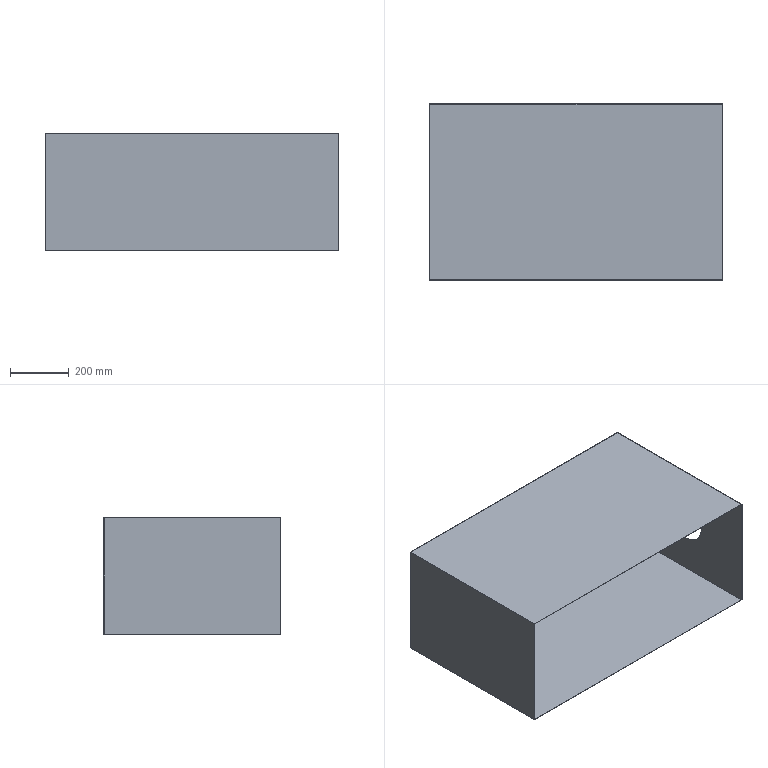Part | SolidWorks | features Cut 1, Extrusion 1, ICE 1 | 1 solid | 13 faces | box 1000 x 600 x 400 mm | volume 2057133 mm3 | plane 11 | cylinder 2 | commonest cylinder face diameters 150 x2
STEP:
#1=CARTESIAN_POINT('',(499.,270.,75.));
#2=VERTEX_POINT('',#1);
#3=CARTESIAN_POINT('',(499.,270.,-75.));
#4=VERTEX_POINT('',#3);
#5=CARTESIAN_POINT('',(499.,270.,0.));
#6=DIRECTION('',(1.,0.,0.));
#7=DIRECTION('',(0.,0.,-1.));
#8=AXIS2_PLACEMENT_3D('',#5,#6,#7);
#9=CIRCLE('',#8,75.);
#10=EDGE_CURVE('',#2,#4,#9,.T.);
#11=ORIENTED_EDGE('',*,*,#10,.F.);
#12=CARTESIAN_POINT('',(500.,270.,75.));
#13=VERTEX_POINT('',#12);
#14=CARTESIAN_POINT('',(450.,270.,75.));
#15=DIRECTION('',(1.,0.,0.));
#16=VECTOR('',#15,1000.);
#17=LINE('',#14,#16);
#18=EDGE_CURVE('',#2,#13,#17,.T.);
#19=ORIENTED_EDGE('',*,*,#18,.T.);
#20=CARTESIAN_POINT('',(500.,270.,-75.));
#21=VERTEX_POINT('',#20);
#22=CARTESIAN_POINT('',(500.,270.,0.));
#23=DIRECTION('',(1.,0.,0.));
#24=DIRECTION('',(0.,0.,-1.));
#25=AXIS2_PLACEMENT_3D('',#22,#23,#24);
#26=CIRCLE('',#25,75.);
#27=EDGE_CURVE('',#13,#21,#26,.T.);
#28=ORIENTED_EDGE('',*,*,#27,.T.);
#29=CARTESIAN_POINT('',(450.,270.,-75.));
#30=DIRECTION('',(1.,0.,0.));
#31=VECTOR('',#30,1000.);
#32=LINE('',#29,#31);
#33=EDGE_CURVE('',#4,#21,#32,.T.);
#34=ORIENTED_EDGE('',*,*,#33,.F.);
#35=EDGE_LOOP('',(#11,#19,#28,#34));
#36=FACE_OUTER_BOUND('',#35,.T.);
#37=CARTESIAN_POINT('',(450.,270.,0.));
#38=DIRECTION('',(1.,0.,0.));
#39=DIRECTION('',(0.,0.,-1.));
#40=AXIS2_PLACEMENT_3D('',#37,#38,#39);
#41=CYLINDRICAL_SURFACE('',#40,75.);
#42=ADVANCED_FACE('',(#36),#41,.F.);
#43=CARTESIAN_POINT('',(500.,270.,0.));
#44=DIRECTION('',(1.,0.,0.));
#45=DIRECTION('',(0.,0.,-1.));
#46=AXIS2_PLACEMENT_3D('',#43,#44,#45);
#47=CIRCLE('',#46,75.);
#48=EDGE_CURVE('',#21,#13,#47,.T.);
#49=ORIENTED_EDGE('',*,*,#48,.F.);
#50=ORIENTED_EDGE('',*,*,#27,.F.);
#51=EDGE_LOOP('',(#49,#50));
#52=FACE_BOUND('',#51,.T.);
#53=CARTESIAN_POINT('',(500.,0.,200.));
#54=VERTEX_POINT('',#53);
#55=CARTESIAN_POINT('',(500.,0.,-200.));
#56=VERTEX_POINT('',#55);
#57=CARTESIAN_POINT('',(500.,0.,-200.));
#58=DIRECTION('',(0.,0.,-1.));
#59=VECTOR('',#58,1000.);
#60=LINE('',#57,#59);
#61=EDGE_CURVE('',#54,#56,#60,.T.);
#62=ORIENTED_EDGE('',*,*,#61,.T.);
#63=CARTESIAN_POINT('',(500.,600.,-200.));
#64=VERTEX_POINT('',#63);
#65=CARTESIAN_POINT('',(500.,600.,-200.));
#66=DIRECTION('',(0.,-1.,0.));
#67=VECTOR('',#66,1000.);
#68=LINE('',#65,#67);
#69=EDGE_CURVE('',#64,#56,#68,.T.);
#70=ORIENTED_EDGE('',*,*,#69,.F.);
#71=CARTESIAN_POINT('',(500.,600.,200.));
#72=VERTEX_POINT('',#71);
#73=CARTESIAN_POINT('',(500.,600.,-200.));
#74=DIRECTION('',(0.,0.,-1.));
#75=VECTOR('',#74,1000.);
#76=LINE('',#73,#75);
#77=EDGE_CURVE('',#72,#64,#76,.T.);
#78=ORIENTED_EDGE('',*,*,#77,.F.);
#79=CARTESIAN_POINT('',(500.,600.,200.));
#80=DIRECTION('',(0.,-1.,0.));
#81=VECTOR('',#80,1000.);
#82=LINE('',#79,#81);
#83=EDGE_CURVE('',#72,#54,#82,.T.);
#84=ORIENTED_EDGE('',*,*,#83,.T.);
#85=EDGE_LOOP('',(#62,#70,#78,#84));
#86=FACE_OUTER_BOUND('',#85,.T.);
#87=CARTESIAN_POINT('',(500.,600.,-200.));
#88=DIRECTION('',(-1.,0.,0.));
#89=DIRECTION('',(0.,0.,1.));
#90=AXIS2_PLACEMENT_3D('',#87,#88,#89);
#91=PLANE('',#90);
#92=ADVANCED_FACE('',(#52,#86),#91,.F.);
#93=CARTESIAN_POINT('',(-500.,0.,-200.));
#94=VERTEX_POINT('',#93);
#95=CARTESIAN_POINT('',(-500.,0.,-200.));
#96=DIRECTION('',(-1.,0.,0.));
#97=VECTOR('',#96,1000.);
#98=LINE('',#95,#97);
#99=EDGE_CURVE('',#56,#94,#98,.T.);
#100=ORIENTED_EDGE('',*,*,#99,.T.);
#101=CARTESIAN_POINT('',(-500.,600.,-200.));
#102=VERTEX_POINT('',#101);
#103=CARTESIAN_POINT('',(-500.,600.,-200.));
#104=DIRECTION('',(0.,-1.,0.));
#105=VECTOR('',#104,1000.);
#106=LINE('',#103,#105);
#107=EDGE_CURVE('',#102,#94,#106,.T.);
#108=ORIENTED_EDGE('',*,*,#107,.F.);
#109=CARTESIAN_POINT('',(-500.,600.,-200.));
#110=DIRECTION('',(-1.,0.,0.));
#111=VECTOR('',#110,1000.);
#112=LINE('',#109,#111);
#113=EDGE_CURVE('',#64,#102,#112,.T.);
#114=ORIENTED_EDGE('',*,*,#113,.F.);
#115=ORIENTED_EDGE('',*,*,#69,.T.);
#116=EDGE_LOOP('',(#100,#108,#114,#115));
#117=FACE_OUTER_BOUND('',#116,.T.);
#118=CARTESIAN_POINT('',(-500.,600.,-200.));
#119=DIRECTION('',(0.,0.,1.));
#120=DIRECTION('',(1.,0.,0.));
#121=AXIS2_PLACEMENT_3D('',#118,#119,#120);
#122=PLANE('',#121);
#123=ADVANCED_FACE('',(#117),#122,.F.);
#124=CARTESIAN_POINT('',(-500.,0.,200.));
#125=VERTEX_POINT('',#124);
#126=CARTESIAN_POINT('',(-500.,0.,-200.));
#127=DIRECTION('',(0.,0.,1.));
#128=VECTOR('',#127,1000.);
#129=LINE('',#126,#128);
#130=EDGE_CURVE('',#94,#125,#129,.T.);
#131=ORIENTED_EDGE('',*,*,#130,.T.);
#132=CARTESIAN_POINT('',(-500.,600.,200.));
#133=VERTEX_POINT('',#132);
#134=CARTESIAN_POINT('',(-500.,600.,200.));
#135=DIRECTION('',(0.,-1.,0.));
#136=VECTOR('',#135,1000.);
#137=LINE('',#134,#136);
#138=EDGE_CURVE('',#133,#125,#137,.T.);
#139=ORIENTED_EDGE('',*,*,#138,.F.);
#140=CARTESIAN_POINT('',(-500.,600.,-200.));
#141=DIRECTION('',(0.,0.,1.));
#142=VECTOR('',#141,1000.);
#143=LINE('',#140,#142);
#144=EDGE_CURVE('',#102,#133,#143,.T.);
#145=ORIENTED_EDGE('',*,*,#144,.F.);
#146=ORIENTED_EDGE('',*,*,#107,.T.);
#147=EDGE_LOOP('',(#131,#139,#145,#146));
#148=FACE_OUTER_BOUND('',#147,.T.);
#149=CARTESIAN_POINT('',(-500.,600.,-200.));
#150=DIRECTION('',(1.,0.,0.));
#151=DIRECTION('',(0.,0.,-1.));
#152=AXIS2_PLACEMENT_3D('',#149,#150,#151);
#153=PLANE('',#152);
#154=ADVANCED_FACE('',(#148),#153,.F.);
#155=CARTESIAN_POINT('',(-500.,0.,200.));
#156=DIRECTION('',(1.,0.,0.));
#157=VECTOR('',#156,1000.);
#158=LINE('',#155,#157);
#159=EDGE_CURVE('',#125,#54,#158,.T.);
#160=ORIENTED_EDGE('',*,*,#159,.T.);
#161=ORIENTED_EDGE('',*,*,#83,.F.);
#162=CARTESIAN_POINT('',(-500.,600.,200.));
#163=DIRECTION('',(1.,0.,0.));
#164=VECTOR('',#163,1000.);
#165=LINE('',#162,#164);
#166=EDGE_CURVE('',#133,#72,#165,.T.);
#167=ORIENTED_EDGE('',*,*,#166,.F.);
#168=ORIENTED_EDGE('',*,*,#138,.T.);
#169=EDGE_LOOP('',(#160,#161,#167,#168));
#170=FACE_OUTER_BOUND('',#169,.T.);
#171=CARTESIAN_POINT('',(-500.,600.,200.));
#172=DIRECTION('',(0.,0.,-1.));
#173=DIRECTION('',(-1.,0.,0.));
#174=AXIS2_PLACEMENT_3D('',#171,#172,#173);
#175=PLANE('',#174);
#176=ADVANCED_FACE('',(#170),#175,.F.);
#177=ORIENTED_EDGE('',*,*,#77,.T.);
#178=ORIENTED_EDGE('',*,*,#113,.T.);
#179=ORIENTED_EDGE('',*,*,#144,.T.);
#180=ORIENTED_EDGE('',*,*,#166,.T.);
#181=EDGE_LOOP('',(#177,#178,#179,#180));
#182=FACE_OUTER_BOUND('',#181,.T.);
#183=CARTESIAN_POINT('',(0.,600.,0.));
#184=DIRECTION('',(0.,1.,0.));
#185=DIRECTION('',(0.,0.,1.));
#186=AXIS2_PLACEMENT_3D('',#183,#184,#185);
#187=PLANE('',#186);
#188=ADVANCED_FACE('',(#182),#187,.T.);
#189=CARTESIAN_POINT('',(499.,0.,199.));
#190=VERTEX_POINT('',#189);
#191=CARTESIAN_POINT('',(-499.,0.,199.));
#192=VERTEX_POINT('',#191);
#193=CARTESIAN_POINT('',(-499.,0.,199.));
#194=DIRECTION('',(-1.,0.,0.));
#195=VECTOR('',#194,1000.);
#196=LINE('',#193,#195);
#197=EDGE_CURVE('',#190,#192,#196,.T.);
#198=ORIENTED_EDGE('',*,*,#197,.F.);
#199=CARTESIAN_POINT('',(499.,0.,-199.));
#200=VERTEX_POINT('',#199);
#201=CARTESIAN_POINT('',(499.,0.,-199.));
#202=DIRECTION('',(0.,0.,1.));
#203=VECTOR('',#202,1000.);
#204=LINE('',#201,#203);
#205=EDGE_CURVE('',#200,#190,#204,.T.);
#206=ORIENTED_EDGE('',*,*,#205,.F.);
#207=CARTESIAN_POINT('',(-499.,0.,-199.));
#208=VERTEX_POINT('',#207);
#209=CARTESIAN_POINT('',(-499.,0.,-199.));
#210=DIRECTION('',(1.,0.,0.));
#211=VECTOR('',#210,1000.);
#212=LINE('',#209,#211);
#213=EDGE_CURVE('',#208,#200,#212,.T.);
#214=ORIENTED_EDGE('',*,*,#213,.F.);
#215=CARTESIAN_POINT('',(-499.,0.,-199.));
#216=DIRECTION('',(0.,0.,-1.));
#217=VECTOR('',#216,1000.);
#218=LINE('',#215,#217);
#219=EDGE_CURVE('',#192,#208,#218,.T.);
#220=ORIENTED_EDGE('',*,*,#219,.F.);
#221=EDGE_LOOP('',(#198,#206,#214,#220));
#222=FACE_BOUND('',#221,.T.);
#223=ORIENTED_EDGE('',*,*,#61,.F.);
#224=ORIENTED_EDGE('',*,*,#159,.F.);
#225=ORIENTED_EDGE('',*,*,#130,.F.);
#226=ORIENTED_EDGE('',*,*,#99,.F.);
#227=EDGE_LOOP('',(#223,#224,#225,#226));
#228=FACE_OUTER_BOUND('',#227,.T.);
#229=CARTESIAN_POINT('',(0.,0.,0.));
#230=DIRECTION('',(0.,1.,0.));
#231=DIRECTION('',(0.,0.,1.));
#232=AXIS2_PLACEMENT_3D('',#229,#230,#231);
#233=PLANE('',#232);
#234=ADVANCED_FACE('',(#222,#228),#233,.F.);
#235=CARTESIAN_POINT('',(499.,270.,0.));
#236=DIRECTION('',(1.,0.,0.));
#237=DIRECTION('',(0.,0.,-1.));
#238=AXIS2_PLACEMENT_3D('',#235,#236,#237);
#239=CIRCLE('',#238,75.);
#240=EDGE_CURVE('',#4,#2,#239,.T.);
#241=ORIENTED_EDGE('',*,*,#240,.T.);
#242=ORIENTED_EDGE('',*,*,#10,.T.);
#243=EDGE_LOOP('',(#241,#242));
#244=FACE_BOUND('',#243,.T.);
#245=ORIENTED_EDGE('',*,*,#205,.T.);
#246=CARTESIAN_POINT('',(499.,599.,199.));
#247=VERTEX_POINT('',#246);
#248=CARTESIAN_POINT('',(499.,599.,199.));
#249=DIRECTION('',(0.,-1.,0.));
#250=VECTOR('',#249,1000.);
#251=LINE('',#248,#250);
#252=EDGE_CURVE('',#247,#190,#251,.T.);
#253=ORIENTED_EDGE('',*,*,#252,.F.);
#254=CARTESIAN_POINT('',(499.,599.,-199.));
#255=VERTEX_POINT('',#254);
#256=CARTESIAN_POINT('',(499.,599.,-199.));
#257=DIRECTION('',(0.,0.,1.));
#258=VECTOR('',#257,1000.);
#259=LINE('',#256,#258);
#260=EDGE_CURVE('',#255,#247,#259,.T.);
#261=ORIENTED_EDGE('',*,*,#260,.F.);
#262=CARTESIAN_POINT('',(499.,599.,-199.));
#263=DIRECTION('',(0.,-1.,0.));
#264=VECTOR('',#263,1000.);
#265=LINE('',#262,#264);
#266=EDGE_CURVE('',#255,#200,#265,.T.);
#267=ORIENTED_EDGE('',*,*,#266,.T.);
#268=EDGE_LOOP('',(#245,#253,#261,#267));
#269=FACE_OUTER_BOUND('',#268,.T.);
#270=CARTESIAN_POINT('',(499.,599.,-199.));
#271=DIRECTION('',(1.,0.,0.));
#272=DIRECTION('',(0.,0.,-1.));
#273=AXIS2_PLACEMENT_3D('',#270,#271,#272);
#274=PLANE('',#273);
#275=ADVANCED_FACE('',(#244,#269),#274,.F.);
#276=ORIENTED_EDGE('',*,*,#213,.T.);
#277=ORIENTED_EDGE('',*,*,#266,.F.);
#278=CARTESIAN_POINT('',(-499.,599.,-199.));
#279=VERTEX_POINT('',#278);
#280=CARTESIAN_POINT('',(-499.,599.,-199.));
#281=DIRECTION('',(1.,0.,0.));
#282=VECTOR('',#281,1000.);
#283=LINE('',#280,#282);
#284=EDGE_CURVE('',#279,#255,#283,.T.);
#285=ORIENTED_EDGE('',*,*,#284,.F.);
#286=CARTESIAN_POINT('',(-499.,599.,-199.));
#287=DIRECTION('',(0.,-1.,0.));
#288=VECTOR('',#287,1000.);
#289=LINE('',#286,#288);
#290=EDGE_CURVE('',#279,#208,#289,.T.);
#291=ORIENTED_EDGE('',*,*,#290,.T.);
#292=EDGE_LOOP('',(#276,#277,#285,#291));
#293=FACE_OUTER_BOUND('',#292,.T.);
#294=CARTESIAN_POINT('',(-499.,599.,-199.));
#295=DIRECTION('',(0.,0.,-1.));
#296=DIRECTION('',(-1.,0.,0.));
#297=AXIS2_PLACEMENT_3D('',#294,#295,#296);
#298=PLANE('',#297);
#299=ADVANCED_FACE('',(#293),#298,.F.);
#300=ORIENTED_EDGE('',*,*,#219,.T.);
#301=ORIENTED_EDGE('',*,*,#290,.F.);
#302=CARTESIAN_POINT('',(-499.,599.,199.));
#303=VERTEX_POINT('',#302);
#304=CARTESIAN_POINT('',(-499.,599.,-199.));
#305=DIRECTION('',(0.,0.,-1.));
#306=VECTOR('',#305,1000.);
#307=LINE('',#304,#306);
#308=EDGE_CURVE('',#303,#279,#307,.T.);
#309=ORIENTED_EDGE('',*,*,#308,.F.);
#310=CARTESIAN_POINT('',(-499.,599.,199.));
#311=DIRECTION('',(0.,-1.,0.));
#312=VECTOR('',#311,1000.);
#313=LINE('',#310,#312);
#314=EDGE_CURVE('',#303,#192,#313,.T.);
#315=ORIENTED_EDGE('',*,*,#314,.T.);
#316=EDGE_LOOP('',(#300,#301,#309,#315));
#317=FACE_OUTER_BOUND('',#316,.T.);
#318=CARTESIAN_POINT('',(-499.,599.,-199.));
#319=DIRECTION('',(-1.,0.,0.));
#320=DIRECTION('',(0.,0.,1.));
#321=AXIS2_PLACEMENT_3D('',#318,#319,#320);
#322=PLANE('',#321);
#323=ADVANCED_FACE('',(#317),#322,.F.);
#324=ORIENTED_EDGE('',*,*,#197,.T.);
#325=ORIENTED_EDGE('',*,*,#314,.F.);
#326=CARTESIAN_POINT('',(-499.,599.,199.));
#327=DIRECTION('',(-1.,0.,0.));
#328=VECTOR('',#327,1000.);
#329=LINE('',#326,#328);
#330=EDGE_CURVE('',#247,#303,#329,.T.);
#331=ORIENTED_EDGE('',*,*,#330,.F.);
#332=ORIENTED_EDGE('',*,*,#252,.T.);
#333=EDGE_LOOP('',(#324,#325,#331,#332));
#334=FACE_OUTER_BOUND('',#333,.T.);
#335=CARTESIAN_POINT('',(-499.,599.,199.));
#336=DIRECTION('',(0.,0.,1.));
#337=DIRECTION('',(1.,0.,0.));
#338=AXIS2_PLACEMENT_3D('',#335,#336,#337);
#339=PLANE('',#338);
#340=ADVANCED_FACE('',(#334),#339,.F.);
#341=ORIENTED_EDGE('',*,*,#260,.T.);
#342=ORIENTED_EDGE('',*,*,#330,.T.);
#343=ORIENTED_EDGE('',*,*,#308,.T.);
#344=ORIENTED_EDGE('',*,*,#284,.T.);
#345=EDGE_LOOP('',(#341,#342,#343,#344));
#346=FACE_OUTER_BOUND('',#345,.T.);
#347=CARTESIAN_POINT('',(0.,599.,0.));
#348=DIRECTION('',(0.,1.,0.));
#349=DIRECTION('',(0.,0.,1.));
#350=AXIS2_PLACEMENT_3D('',#347,#348,#349);
#351=PLANE('',#350);
#352=ADVANCED_FACE('',(#346),#351,.F.);
#353=ORIENTED_EDGE('',*,*,#18,.F.);
#354=ORIENTED_EDGE('',*,*,#240,.F.);
#355=ORIENTED_EDGE('',*,*,#33,.T.);
#356=ORIENTED_EDGE('',*,*,#48,.T.);
#357=EDGE_LOOP('',(#353,#354,#355,#356));
#358=FACE_OUTER_BOUND('',#357,.T.);
#359=CARTESIAN_POINT('',(450.,270.,0.));
#360=DIRECTION('',(1.,0.,0.));
#361=DIRECTION('',(0.,0.,-1.));
#362=AXIS2_PLACEMENT_3D('',#359,#360,#361);
#363=CYLINDRICAL_SURFACE('',#362,75.);
#364=ADVANCED_FACE('',(#358),#363,.F.);
#365=CLOSED_SHELL('',(#42,#92,#123,#154,#176,#188,#234,#275,#299,#323,#340,#352,#364));
#366=MANIFOLD_SOLID_BREP('',#365);
#367=CARTESIAN_POINT('',(0.,0.,0.));
#368=DIRECTION('',(0.,0.,1.));
#369=DIRECTION('',(1.,0.,0.));
#370=AXIS2_PLACEMENT_3D('',#367,#368,#369);
#371=(LENGTH_UNIT()NAMED_UNIT(*)SI_UNIT(.MILLI.,.METRE.));
#372=UNCERTAINTY_MEASURE_WITH_UNIT(LENGTH_MEASURE(0.00001),#371,'','');
#373=(NAMED_UNIT(*)PLANE_ANGLE_UNIT()SI_UNIT($,.RADIAN.));
#374=(NAMED_UNIT(*)SI_UNIT($,.STERADIAN.)SOLID_ANGLE_UNIT());
#375=(GEOMETRIC_REPRESENTATION_CONTEXT(3)GLOBAL_UNCERTAINTY_ASSIGNED_CONTEXT((#372))GLOBAL_UNIT_ASSIGNED_CONTEXT((#371,#373,#374))REPRESENTATION_CONTEXT('',''));
#376=ADVANCED_BREP_SHAPE_REPRESENTATION('',(#366,#370),#375);